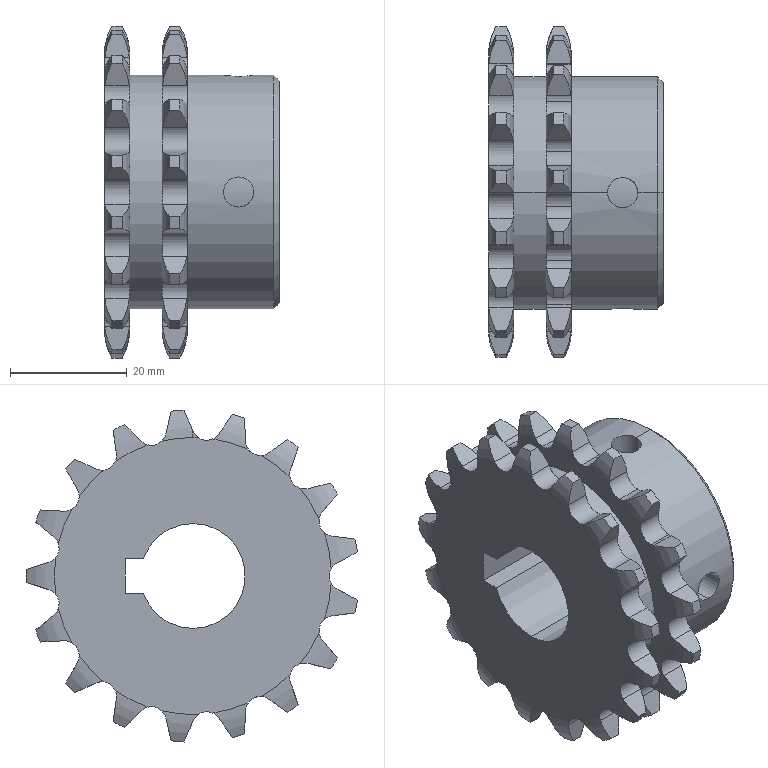Part | SolidWorks | features BaseBody 1 | 1 solid | 243 faces | box 30 x 56.698 x 56.919 mm | volume 35879 mm3 | cylinder 93 | plane 76 | spline 72 | cone 2 | commonest cylinder face diameters 5.08 x46 57 x34 5.188 x4 40 x4 18 x3 28.265 x2